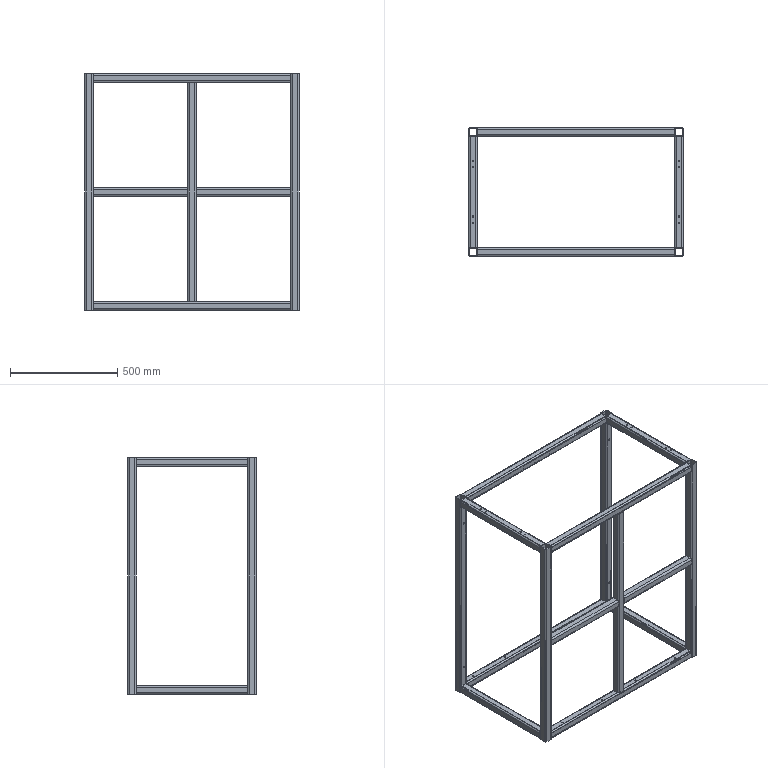Part | STEP file | 15 solids | 412 faces | box 1000 x 600 x 1100 mm | volume 7334551 mm3 | cylinder 214 | plane 142 | cone 56 | commonest cylinder face diameters 16 x60 8 x52 5 x36 2.5 x32 6.8 x32 3.3 x2